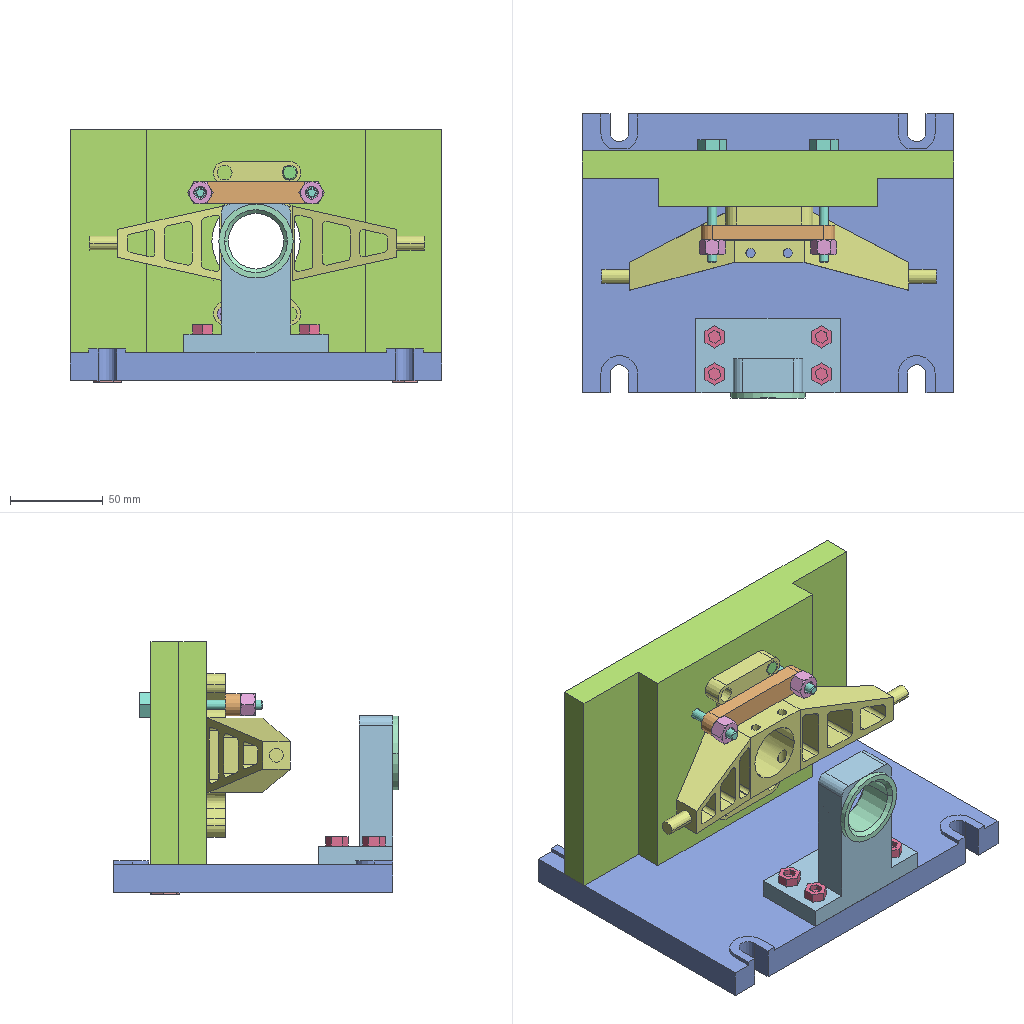Assembly | NX | 11 different items | 18 placed | box 200 x 153 x 136 mm
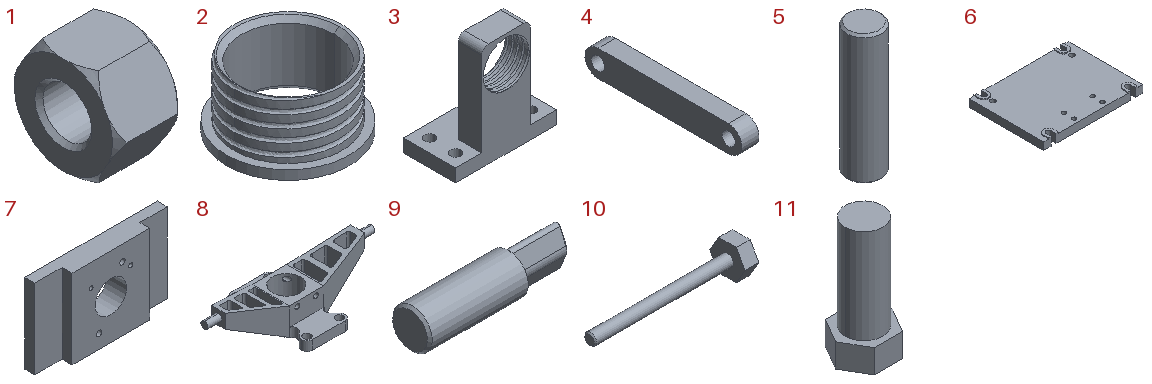Parts list (item | quantity | size | volume | features):
1 | x2 | 8 x 13.765 x 11.921 mm | 747.808 mm3 | features DATUM_CSYS 4, EXTRUDE 3, OFFSET_REGION 3, SKETCH 3, CHAMFER 2
2 | x1 | - | 5444 mm3 | features SKETCH 3, DATUM_CSYS 2, BREP 1, CHAMFER 1, DATUM_ON_PATH 1, EXTRUDE 1, HELIX 1, VARIATIONAL_SWEEP 1
3 | x1 | - | 58227 mm3 | features SKETCH 3, DATUM_CSYS 2, BREP 1, DATUM_ON_PATH 1, EXTRUDE 1, HELIX 1, VARIATIONAL_SWEEP 1
4 | x1 | 8 x 72 x 12 mm | 6212 mm3 | features OFFSET_REGION 3, DATUM_CSYS 2, EXTRUDE 1, SKETCH 1
5 | x1 | 8 x 8 x 30 mm | 1502 mm3 | features DATUM_CSYS 2, CHAMFER 1, EXTRUDE 1, SKETCH 1
6 | x1 | 200 x 150 x 17 mm | 435629 mm3 | features DATUM_CSYS 9, EXTRUDE 9, SKETCH 9, OFFSET_REGION 5, BREP 1, DELETE FACE 1
7 | x1 | 200 x 30 x 120 mm | 506738 mm3 | features DATUM_CSYS 10, EXTRUDE 10, SKETCH 10, OFFSET_REGION 5, BREP 1, DELETE FACE 1
8 | x1 | 180 x 88 x 45 mm | 75635 mm3 | features BREP 2
9 | x1 | 30 x 8 x 8 mm | 1212 mm3 | features DATUM_CSYS 3, BLEND 2, EXTRUDE 2, SKETCH 2, CHAMFER 1
10 | x4 | 66 x 15.381 x 13.321 mm | 1888 mm3 | features DATUM_CSYS 4, EXTRUDE 3, OFFSET_REGION 3, SKETCH 3, CHAMFER 1
11 | x4 | 12 x 10.392 x 25 mm | 1379 mm3 | features BREP 1, DATUM_CSYS 1, EXTRUDE 1, SKETCH 1
Mates (type | each side: item.copy, entity, surface, feature):
Touch | assembly face cylinder Extrude(1) | 6.1 face cylinder Extrude(16)
Concentric | assembly edge | 6.1
Touch | assembly face plane Extrude(2) | 6.1 face plane Body(0)
Concentric | 10.1 edge | 6.1 edge | 2 times